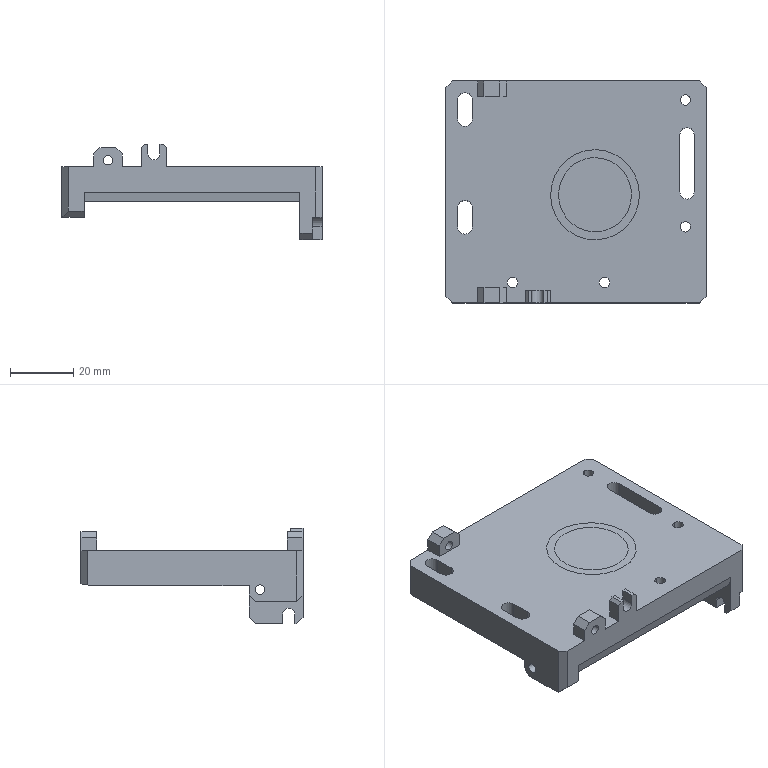NC program | NX | posted with a generic post | part box 82 x 70 x 30 mm
Lines 3883 to 5501 of 5501:
(FIXED_CONTOUR_COPY_1 , TOOL : R0.75)
N7734 T12 M6
N7736 G54
N7738 G17 G0 G90 X-35.125 Y13.063 B0. C0. S9500 M3
N7740 G43 Z30. H12
N7742 Z3.
N7744 G94 G1 Z-3.867 F1000.
N7746 X-35.098 Y13.111
N7748 X-35.049 Y13.139
N7750 X-34.995 Y13.138
N7752 X-34.959 Z-3.87 F2000.
N7754 X-34.909
N7756 X-34.892 Y13.145 Z-3.813
N7758 X-34.891 Y13.147 Z-3.801
N7760 X-34.708 Y13.148 Z-0.878
N7762 X-34.694 Z-0.85
N7764 X-31.316
N7766 X-31.288 Z-0.958
N7768 X-31.114 Y13.147 Z-3.801
N7770 X-31.092 Y13.138 Z-3.869
N7772 X-31.008 Z-3.891
N7774 X-31.092 Z-3.869
N7776 X-31.105
N7778 X-31.214 Y13.147 Z-3.801
N7780 X-31.384 Y13.148 Z-1.013
N7782 X-31.441 Z-0.95
N7784 X-34.599
N7786 X-34.631 Z-1.249
N7788 X-34.792 Y13.146 Z-3.807
N7790 X-34.809 Y13.138 Z-3.87
N7792 X-34.959
N7794 X-34.995 Z-3.868
N7796 X-34.959 Z-3.871
N7798 X-34.808 Z-3.87
N7800 X-34.692 Y13.145 Z-3.812
N7802 X-34.691 Y13.147 Z-3.801
N7804 X-34.531 Y13.148 Z-1.258
N7806 X-34.512 Z-1.077
N7808 X-34.486 Z-1.05
N7810 X-31.491
N7812 X-31.358 Y13.147 Z-3.081
N7814 X-31.314 Z-3.801
N7816 X-31.163 Y13.138 Z-3.869
N7818 X-31.092
N7820 X-31.008 Z-3.891
N7822 X-31.092 Z-3.869
N7824 X-31.33
N7826 X-31.414 Y13.147 Z-3.801
N7828 X-31.569 Y13.148 Z-1.378
N7830 X-31.595 Z-1.15
N7832 X-34.4
N7834 X-34.421 Z-1.169
N7836 X-34.431 Z-1.265
N7838 X-34.591 Y13.147 Z-3.801
N7840 X-34.599 Y13.141 Z-3.85
N7842 X-34.67 Y13.138 Z-3.87
N7844 X-34.959 Z-3.871
N7846 X-34.995 Z-3.868
N7848 X-34.959 Z-3.871
N7850 X-34.569
N7852 X-34.492 Y13.144 Z-3.819
N7854 X-34.491 Y13.147 Z-3.801
N7856 X-34.337 Y13.148 Z-1.352
N7858 X-34.318 Z-1.25
N7860 X-31.725
N7862 X-31.679 Z-1.3
N7864 X-31.547 Y13.147 Z-3.299
N7866 X-31.514 Z-3.801
N7868 X-31.379 Y13.138 Z-3.87
N7870 X-31.092
N7872 X-31.008 Z-3.891
N7874 X-31.092 Z-3.87
N7876 X-31.569
N7878 X-31.615 Y13.147 Z-3.801
N7880 X-31.765 Y13.148 Z-1.516
N7882 X-31.778 Z-1.35
N7884 X-34.224
N7886 X-34.249 Z-1.544
N7888 X-34.39 Y13.147 Z-3.801
N7890 X-34.393 Y13.143 Z-3.828
N7892 X-34.431 Y13.138 Z-3.871
N7894 X-34.959
N7896 X-34.995 Z-3.869
N7898 X-34.959 Z-3.871
N7900 X-34.33
N7902 X-34.291 Y13.145 Z-3.814
N7904 X-34.29 Y13.147 Z-3.801
N7906 X-34.149 Y13.148 Z-1.555
N7908 X-34.137 Z-1.458
N7910 X-33.954 Z-1.45
N7912 X-31.9
N7914 X-31.847 Z-1.782
N7916 X-31.715 Y13.147 Z-3.801
N7918 X-31.595 Y13.138 Z-3.87
N7920 X-31.092
N7922 X-31.008 Z-3.892
N7924 X-31.092 Z-3.87
N7926 X-31.707
N7928 X-31.807 Y13.142 Z-3.839
N7930 X-31.815 Y13.147 Z-3.801
N7932 X-31.916 Z-2.261
N7934 X-31.981 Y13.148 Z-1.572
N7936 X-31.985 Z-1.55
N7938 X-33.954
N7940 X-34.042 Z-1.554
N7942 X-34.085 Z-2.124
N7944 X-34.19 Y13.147 Z-3.801
N7946 X-34.193 Y13.143 Z-3.832
N7948 X-34.33 Y13.138 Z-3.871
N7950 X-34.96 Z-3.872
N7952 X-34.995 Z-3.869
N7954 X-34.96 Z-3.872
N7956 X-34.123 Z-3.871
N7958 X-34.099 Y13.139 Z-3.866
N7960 X-34.09 Y13.147 Z-3.8
N7962 X-34.006 Y13.148 Z-2.468
N7964 X-33.954 Z-1.726
N7966 X-33.944 Z-1.65
N7968 X-32.088
N7970 X-32.046 Z-1.95
N7972 X-31.97 Y13.147 Z-2.971
N7974 X-31.915 Z-3.801
N7976 X-31.812 Y13.138 Z-3.871
N7978 X-31.092 Z-3.87
N7980 X-31.008 Z-3.892
N7982 X-31.092 Z-3.871
N7984 X-31.869
N7986 X-32.016 Y13.147 Z-3.801
N7988 X-32.059 Z-3.136
N7990 X-32.088 Z-2.729
N7992 X-32.16 Y13.148 Z-1.856
N7994 X-32.186 Z-1.75
N7996 X-33.855
N7998 X-33.951 Z-3.192
N8000 X-33.99 Y13.147 Z-3.801
N8002 X-33.991 Y13.145 Z-3.818
N8004 X-34.091 Y13.138 Z-3.872
N8006 X-34.96
N8008 X-34.995 Z-3.869
N8010 Z-3.871
N8012 X-34.961 Z-3.874
N8014 X-33.954 Z-3.873
N8016 X-33.889 Y13.147 Z-3.801
N8018 X-33.767 Y13.148 Z-1.943
N8020 X-33.754 Z-1.85
N8022 X-32.273
N8024 X-32.258 Z-1.888
N8026 X-32.232 Z-2.203
N8028 X-32.116 Y13.147 Z-3.801
N8030 X-32.046 Y13.138 Z-3.873
N8032 X-31.092
N8034 X-31.008 Z-3.894
N8036 Z-3.896
N8038 X-31.092 Z-3.875
N8040 X-32.084
N8042 X-32.216 Y13.147 Z-3.801
N8044 X-32.284 Z-2.859
N8046 X-32.357 Y13.148 Z-1.95
N8048 X-33.657
N8050 X-33.677 Z-2.085
N8052 X-33.789 Y13.147 Z-3.8
N8054 X-33.792 Y13.144 Z-3.824
N8056 X-33.954 Y13.138 Z-3.875
N8058 X-34.963 Z-3.876
N8060 X-34.995 Z-3.874
N8062 X-34.963 Z-3.877
N8064 X-33.716 Z-3.876
N8066 X-33.691 Y13.144 Z-3.818
N8068 X-33.689 Y13.147 Z-3.801
N8070 X-33.577 Y13.148 Z-2.096
N8072 X-33.546 Z-2.05
N8074 X-32.45
N8076 X-32.357 Y13.147 Z-3.234
N8078 X-32.316 Z-3.801
N8080 X-32.284 Y13.138 Z-3.874
N8082 X-31.906 Z-3.875
N8084 X-31.092
N8086 X-31.008 Z-3.897
N8088 X-31.092 Z-3.876
N8090 X-32.302
N8092 X-32.417 Y13.147 Z-3.801
N8094 X-32.496 Z-2.741
N8096 X-32.539 Y13.148 Z-2.183
N8098 X-32.588 Z-2.15
N8100 X-33.478
N8102 X-33.536 Y13.147 Z-3.002
N8104 X-33.589 Y13.145 Z-3.81
N8106 X-33.607 Y13.138 Z-3.876
N8108 X-34.963 Y13.137 Z-3.877
N8110 X-34.995 Z-3.875
N8112 X-34.964 Z-3.878
N8114 X-33.606 Z-3.877
N8116 X-33.489 Y13.146 Z-3.808
N8118 X-33.385 Y13.147 Z-2.256
N8120 X-33.36 Z-2.25
N8122 X-32.644
N8124 X-32.53 Z-3.617
N8126 X-32.517 Z-3.801
N8128 X-32.356 Y13.138 Z-3.876
N8130 X-31.092
N8132 X-31.008 Z-3.898
N8134 X-31.092 Y13.137 Z-3.877
N8136 X-32.523
N8138 X-32.617 Y13.147 Z-3.801
N8140 X-32.724 Z-2.491
N8142 X-32.74 Z-2.35
N8144 X-33.267
N8146 X-33.294 Z-2.389
N8148 X-33.388 Z-3.801
N8150 X-33.4 Y13.14 Z-3.854
N8152 X-33.477 Y13.137 Z-3.877
N8154 X-34.964 Z-3.878
N8156 X-34.995 Z-3.876
N8158 X-34.965 Z-3.879
N8160 X-33.366 Z-3.878
N8162 X-33.29 Y13.145 Z-3.818
N8164 X-33.288 Y13.147 Z-3.801
N8166 X-33.205 Z-2.553
N8168 X-33.193 Z-2.45
N8170 X-32.841
N8172 X-32.802 Z-2.768
N8174 X-32.717 Z-3.801
N8176 X-32.573 Y13.137 Z-3.877
N8178 X-31.092
N8180 X-31.008 Z-3.899
N8182 X-31.092 Z-3.878
N8184 X-32.761
N8186 X-32.818 Y13.147 Z-3.801
N8188 X-32.906 Z-2.741
N8190 X-32.931 Z-2.55
N8192 X-33.098
N8194 X-33.128 Z-2.902
N8196 X-33.188 Z-3.801
N8198 X-33.191 Y13.143 Z-3.834
N8200 X-33.239 Y13.137 Z-3.878
N8202 X-34.965 Z-3.879
N8204 X-34.995 Z-3.877
N8206 X-34.965 Z-3.88
N8208 X-33.126 Z-3.879
N8210 X-33.089 Y13.145 Z-3.816
N8212 X-33.088 Y13.147 Z-3.801
N8214 X-33.033 Z-2.97
N8216 X-33.011 Z-2.71
N8218 X-33. Z-2.817
N8220 X-32.918 Z-3.801
N8222 X-32.791 Y13.137 Z-3.879
N8224 X-31.092 Z-3.878
N8226 X-31.008 Z-3.9
N8228 X-31.092 Z-3.878
N8230 X-32.791 Z-3.879
N8232 X-32.819 Y13.139 Z-3.862
N8234 X-33.116
N8236 X-33.126 Y13.137 Z-3.879
N8238 X-34.965 Z-3.88
N8240 X-34.995 Z-3.878
N8242 X-34.997 Y13.127 Z-3.962
N8244 X-31.092 Z-3.961
N8246 X-31.085 Z-3.962
N8248 X-31.007 Z-3.963
N8250 X-31.005 Y13.099 Z-4.058
N8252 X-31.569 Z-4.056
N8254 X-34.909 Z-4.057
N8256 X-34.999 Z-4.058
N8258 X-35. Y13.07 Z-4.154
N8260 X-34.192 Z-4.152
N8262 X-31.002 Z-4.153
N8264 Y13.053 Z-4.194
N8266 X-31.001 Y13.028 Z-4.241
N8268 X-31.012 Z-4.239
N8270 X-31.051 Z-4.243
N8272 X-34.95 Z-4.244
N8274 X-34.989 Z-4.257
N8276 X-34.999 Z-4.259
N8278 X-35. Y12.985 Z-4.338
N8280 X-34.909 Z-4.326
N8282 X-31.092
N8284 X-31.055 Z-4.322
N8286 X-31.001 Z-4.334
N8288 X-31. Y12.97 Z-4.365
N8290 X-31.001 Y12.949 Z-4.401
N8292 Y12.934 Z-4.418
N8294 X-31.078 Z-4.411
N8296 X-34.924 Y12.933
N8298 X-35. Z-4.418
N8300 Y12.87 Z-4.49
N8302 X-34.67 Z-4.488
N8304 X-31.013 Z-4.489
N8306 X-31. Z-4.49
N8308 Y12.83 Z-4.538
N8310 Y12.802 Z-4.562
N8312 X-35.
N8314 Y12.73 Z-4.631
N8316 X-34.909 Z-4.626
N8318 X-31.073
N8320 X-31. Z-4.631
N8322 X-31.001 Y12.711 Z-4.649
N8324 Y12.65 Z-4.688
N8326 X-31.03 Z-4.686
N8328 X-34.97
N8330 X-34.999 Z-4.688
N8332 X-35. Y12.593 Z-4.727
N8334 Y12.567 Z-4.741
N8336 X-31.
N8338 Y12.479 Z-4.781
N8340 X-31.087 Z-4.788
N8342 X-34.913 Y12.478
N8344 X-35. Z-4.781
N8346 Y12.387 Z-4.823
N8348 X-31.
N8350 Y12.328 Z-4.843
N8352 Y12.292 Z-4.852
N8354 X-31.092 Z-4.853
N8356 X-34.964 Z-4.854
N8358 X-35. Z-4.852
N8360 Y12.195 Z-4.876
N8362 X-34.951 Z-4.878
N8364 X-31.05
N8366 X-31. Z-4.876
N8368 Y12.119 Z-4.893
N8370 Y12.097 Z-4.894
N8372 X-35.
N8374 Y11.997 Z-4.895
N8376 X-34.911 Z-4.899
N8378 X-31.089
N8380 X-31. Z-4.895
N8382 Y11.897 Z-4.894
N8384 X-35.
N8386 Y11.881 Z-4.893
N8388 Y11.799 Z-4.874
N8390 X-34.909 Z-4.877
N8392 X-31.055
N8394 X-31. Z-4.874
N8396 Y11.703 Z-4.851
N8398 X-31.092 Z-4.852
N8400 X-34.969
N8402 X-35. Z-4.851
N8404 Y11.644 Z-4.835
N8406 Y11.608 Z-4.82
N8408 X-31.
N8410 Y11.517 Z-4.779
N8412 X-31.082 Z-4.785
N8414 X-34.918 Y11.516
N8416 X-35. Z-4.779
N8418 Y11.428 Z-4.738
N8420 X-31. Z-4.739
N8422 Y11.407 Z-4.727
N8424 X-31.001 Y11.345 Z-4.685
N8426 X-31.034 Z-4.683
N8428 X-34.965
N8430 X-34.999 Z-4.685
N8432 X-35. Y11.289 Z-4.649
N8434 Y11.266 Z-4.627
N8436 X-34.909 Z-4.622
N8438 X-31.069
N8440 X-31. Z-4.627
N8442 Y11.193 Z-4.558
N8444 X-35.
N8446 Y11.17 Z-4.538
N8448 Y11.126 Z-4.486
N8450 X-34.909 Z-4.483
N8452 X-31.016 Z-4.484
N8454 X-31. Z-4.486
N8456 X-31.001 Y11.063 Z-4.414
N8458 X-31.08 Z-4.406
N8460 X-34.92
N8462 X-35. Z-4.414
N8464 X-34.999 Y11.051 Z-4.401
N8466 X-35. Y11.029 Z-4.363
N8468 Y11.014 Z-4.332
N8470 X-34.956 Z-4.323
N8472 X-34.909 Z-4.325
N8474 X-31.092
N8476 X-31.054 Z-4.321
N8478 X-31. Z-4.332
N8480 Y10.971 Z-4.24
N8482 X-31.011 Z-4.238
N8484 X-31.05 Z-4.242
N8486 X-34.951
N8488 X-34.962 Z-4.244
N8490 X-35. Z-4.242
N8492 Y10.956 Z-4.214
N8494 Y10.933 Z-4.163
N8496 Y10.929 Z-4.152
N8498 X-34.67 Z-4.15
N8500 X-31.081 Z-4.151
N8502 X-31. Z-4.152
N8504 Y10.9 Z-4.058
N8506 X-31.092 Z-4.055
N8508 X-34.909
N8510 X-34.999 Z-4.057
N8512 X-34.996 Y10.872 Z-3.962
N8514 X-34.909 Z-3.959
N8516 X-31.081 Z-3.96
N8518 X-31.001 Z-3.963
N8520 X-31.002 Y10.859 Z-3.883
N8522 Y10.858 Z-3.867
N8524 X-31.092 Z-3.862
N8526 X-34.909 Z-3.86
N8528 X-34.925 Z-3.862
N8530 X-34.955 Z-3.873
N8532 X-34.994 Z-3.876
N8534 X-34.989 Y10.852 Z-3.776
N8536 X-34.909 Z-3.766
N8538 X-31.08 Z-3.769
N8540 X-31.065 Z-3.781
N8542 X-31.002 Z-3.786
N8544 Y10.85 Z-3.751
N8546 Z-3.686
N8548 X-31.092 Z-3.668
N8550 X-34.913 Y10.851 Z-3.666
N8552 X-34.983 Y10.85 Z-3.674
N8554 X-34.976 Z-3.573
N8556 X-34.917 Z-3.566
N8558 X-31.092 Z-3.568
N8560 X-31.002 Z-3.584
N8562 Z-3.482
N8564 X-31.092 Z-3.468
N8566 X-34.921 Y10.851 Z-3.466
N8568 X-34.97 Y10.85 Z-3.471
N8570 X-34.964 Z-3.37
N8572 X-34.925 Z-3.366
N8574 X-31.092 Z-3.368
N8576 X-31.002 Z-3.381
N8578 Z-3.28
N8580 X-31.092 Z-3.268
N8582 X-34.93 Y10.851 Z-3.266
N8584 X-34.957 Y10.85 Z-3.269
N8586 X-34.951 Z-3.168
N8588 X-34.909 Z-3.166
N8590 X-31.092 Z-3.168
N8592 X-31.002 Z-3.179
N8594 X-31.001 Z-3.078
N8596 X-31.092 Z-3.068
N8598 X-34.945 Z-3.067
N8600 X-34.941 Z-3.012
N8602 X-34.942 Z-2.985
N8604 X-34.94 Y10.849
N8606 X-34.938 Z-2.966
N8608 X-31.092 Y10.85 Z-2.968
N8610 X-31.001 Z-2.977
N8612 Z-2.876
N8614 X-31.092 Z-2.868
N8616 X-34.932 Y10.849 Z-2.866
N8618 X-34.926 Y10.85 Z-2.766
N8620 X-31.092 Z-2.768
N8622 X-31.001 Z-2.776
N8624 Z-2.675
N8626 X-31.092 Z-2.668
N8628 X-34.92 Z-2.666
N8630 X-34.913 Z-2.566
N8632 X-31.092 Z-2.568
N8634 X-31.001 Z-2.575
N8636 Z-2.475
N8638 X-31.092 Z-2.468
N8640 X-34.907 Z-2.466
N8642 X-34.901 Z-2.366
N8644 X-31.092 Z-2.368
N8646 X-31.001 Z-2.374
N8648 Z-2.274
N8650 X-31.092 Z-2.268
N8652 X-34.895 Z-2.266
N8654 X-34.888 Z-2.166
N8656 X-31.092 Z-2.168
N8658 X-31.001 Z-2.174
N8660 Z-2.073
N8662 X-31.092 Z-2.068
N8664 X-34.882 Z-2.066
N8666 X-34.876 Z-1.966
N8668 X-31.092 Z-1.968
N8670 X-31.001 Z-1.973
N8672 Z-1.873
N8674 X-31.092 Z-1.868
N8676 X-34.87 Z-1.866
N8678 X-34.863 Z-1.766
N8680 X-31.092 Z-1.768
N8682 X-31.001 Z-1.773
N8684 Z-1.672
N8686 X-31.092 Z-1.668
N8688 X-34.857 Z-1.666
N8690 X-34.851 Z-1.566
N8692 X-31.092 Z-1.568
N8694 X-31.001 Z-1.572
N8696 Z-1.472
N8698 X-31.092 Z-1.468
N8700 X-34.845 Z-1.466
N8702 X-34.838 Z-1.366
N8704 X-31.092 Z-1.368
N8706 X-31.001 Z-1.372
N8708 Z-1.272
N8710 X-31.092 Z-1.268
N8712 X-34.832 Z-1.266
N8714 X-34.826 Z-1.166
N8716 X-31.092 Z-1.168
N8718 X-31.001 Z-1.171
N8720 X-31. Z-1.071
N8722 X-31.092 Z-1.068
N8724 X-34.82 Z-1.066
N8726 X-34.813 Z-0.966
N8728 X-31.092 Z-0.968
N8730 X-31. Z-0.971
N8732 Z-0.871
N8734 X-31.088 Z-0.868
N8736 X-34.807 Z-0.866
N8738 X-34.801 Z-0.766
N8740 X-31.091 Z-0.768
N8742 X-31. Z-0.771
N8744 X-30.946 Y10.849
N8746 X-30.897 Y10.877
N8748 X-30.87 Y10.924
N8750 Z3.
N8752 G0 Z30.
N8754 M5
(ZLEVEL_PROFILE_1_COPY_1 , TOOL : D3R0.5)
N8756 T05 M6
N8758 G54
N8760 G17 G0 G90 X-35.973 Y16.812 B0. C0. S9500 M3
N8762 G43 Z30. H5
N8764 Z1.429
N8766 G94 G1 Z-0.071 F1000.
N8768 X-35.735 Y16.42
N8770 G3 X-35.472 Y16.275 R0.3
N8772 G1 X-35.35 Y16.278 F2500.
N8774 X-30.55
N8776 X-30.528 Y16.276
N8778 Y16.313 Z-0.106
N8780 Y16.347 Z-0.141
N8782 X-30.55 Y16.349
N8784 X-35.35
N8786 X-35.472 Y16.346
N8788 Y16.384 Z-0.177
N8790 Y16.417 Z-0.212
N8792 X-35. Y16.419
N8794 X-30.55
N8796 X-30.528 Y16.418
N8798 Y16.455 Z-0.247
N8800 Y16.488 Z-0.283
N8802 X-30.55 Y16.49
N8804 X-35.
N8806 X-35.472 Y16.487
N8808 Y16.525 Z-0.318
N8810 Y16.558 Z-0.354
N8812 X-35. Y16.561
N8814 X-30.55
N8816 X-30.528 Y16.559
N8818 Y16.596 Z-0.389
N8820 Y16.63 Z-0.424
N8822 X-30.55 Y16.631
N8824 X-35.
N8826 X-35.472 Y16.629
N8828 Y16.667 Z-0.46
N8830 Y16.699 Z-0.495
N8832 X-35. Y16.702
N8834 X-30.55
N8836 X-30.528 Y16.7
N8838 Y16.737 Z-0.53
N8840 Y16.771 Z-0.566
N8842 X-30.55 Y16.773
N8844 X-35.
N8846 X-35.472 Y16.77
N8848 Y16.808 Z-0.601
N8850 Y16.841 Z-0.636
N8852 X-35. Y16.844
N8854 X-30.55
N8856 X-30.528 Y16.842
N8858 Y16.879 Z-0.672
N8860 Y16.913 Z-0.707
N8862 X-30.55 Y16.914
N8864 X-35.
N8866 X-35.472 Y16.912
N8868 Y16.95 Z-0.742
N8870 Y16.982 Z-0.778
N8872 X-35. Y16.985
N8874 X-30.55
N8876 X-30.528 Y16.983
N8878 Y17.02 Z-0.813
N8880 Y17.054 Z-0.849
N8882 X-30.55 Y17.056
N8884 X-35.
N8886 X-35.472 Y17.053
N8888 Y17.091 Z-0.884
N8890 Y17.124 Z-0.919
N8892 X-35. Y17.126
N8894 X-30.55
N8896 X-30.528 Y17.125
N8898 Y17.162 Z-0.955
N8900 Y17.195 Z-0.99
N8902 X-30.55 Y17.197
N8904 X-35.
N8906 X-35.472 Y17.194
N8908 Y17.232 Z-1.025
N8910 Y17.265 Z-1.061
N8912 X-35. Y17.268
N8914 X-30.55
N8916 X-30.528 Y17.266
N8918 Y17.303 Z-1.096
N8920 Y17.337 Z-1.131
N8922 X-30.55 Y17.338
N8924 X-35.
N8926 X-35.472 Y17.336
N8928 Y17.374 Z-1.167
N8930 Y17.407 Z-1.202
N8932 X-35.35 Y17.409
N8934 X-30.55
N8936 X-30.528 Y17.408
N8938 Y17.445 Z-1.237
N8940 Y17.478 Z-1.273
N8942 X-30.55 Y17.48
N8944 X-35.35
N8946 X-35.472 Y17.477
N8948 Y17.508 Z-1.301
N8950 Y17.534 Z-1.33
N8952 X-35.35 Y17.537
N8954 X-30.55
N8956 X-30.528 Y17.535
N8958 Y17.565 Z-1.358
N8960 Y17.592 Z-1.386
N8962 X-30.55 Y17.594
N8964 X-35.35
N8966 X-35.472 Y17.591
N8968 X-35.419 Y17.648 Z-1.443
N8970 X-35.35 Y17.65
N8972 X-30.538 Y17.649
N8974 G3 X-30.278 Y17.799 R0.3
N8976 G1 X-30.052 Y18.19
N8978 Z0.057
N8980 G0 Z30.
N8982 X-29.99 Y7.198
N8984 Z1.429
N8986 G1 Z-0.071 F1000.
N8988 X-30.258 Y7.593
N8990 G3 X-30.528 Y7.724 R0.3
N8992 G1 X-30.55 Y7.722 F2500.
N8994 X-35.35
N8996 X-35.472 Y7.725
N8998 Y7.687 Z-0.106
N9000 Y7.654 Z-0.141
N9002 X-35.35 Y7.651
N9004 X-30.55
N9006 X-30.528 Y7.653
N9008 Y7.616 Z-0.177
N9010 Y7.582 Z-0.212
N9012 X-30.55 Y7.581
N9014 X-35.
N9016 X-35.472 Y7.583
N9018 Y7.545 Z-0.247
N9020 Y7.513 Z-0.283
N9022 X-35. Y7.51
N9024 X-30.55
N9026 X-30.528 Y7.512
N9028 Y7.475 Z-0.318
N9030 Y7.441 Z-0.354
N9032 X-30.55 Y7.439
N9034 X-35.
N9036 X-35.472 Y7.442
N9038 Y7.404 Z-0.389
N9040 Y7.371 Z-0.424
N9042 X-35. Y7.369
N9044 X-30.55
N9046 X-30.528 Y7.37
N9048 Y7.333 Z-0.46
N9050 Y7.3 Z-0.495
N9052 X-30.55 Y7.298
N9054 X-35.
N9056 X-35.472 Y7.301
N9058 Y7.263 Z-0.53
N9060 Y7.23 Z-0.566
N9062 X-35. Y7.227
N9064 X-30.55
N9066 X-30.528 Y7.229
N9068 Y7.192 Z-0.601
N9070 Y7.158 Z-0.636
N9072 X-30.55 Y7.156
N9074 X-35.
N9076 X-35.472 Y7.159
N9078 Y7.121 Z-0.672
N9080 Y7.088 Z-0.707
N9082 X-35. Y7.086
N9084 X-30.55
N9086 X-30.528 Y7.087
N9088 Y7.05 Z-0.742
N9090 Y7.017 Z-0.778
N9092 X-30.55 Y7.015
N9094 X-35.
N9096 X-35.472 Y7.018
N9098 Y6.98 Z-0.813
N9100 Y6.947 Z-0.849
N9102 X-35. Y6.944
N9104 X-30.55
N9106 X-30.528 Y6.946
N9108 Y6.909 Z-0.884
N9110 Y6.875 Z-0.919
N9112 X-30.55 Y6.874
N9114 X-35.
N9116 X-35.472 Y6.876
N9118 Y6.838 Z-0.955
N9120 Y6.806 Z-0.99
N9122 X-35. Y6.803
N9124 X-30.55
N9126 X-30.528 Y6.805
N9128 Y6.768 Z-1.025
N9130 Y6.734 Z-1.061
N9132 X-30.55 Y6.732
N9134 X-35.
N9136 X-35.472 Y6.735
N9138 Y6.697 Z-1.096
N9140 Y6.664 Z-1.131
N9142 X-35. Y6.662
N9144 X-30.55
N9146 X-30.528 Y6.663
N9148 Y6.626 Z-1.167
N9150 Y6.592 Z-1.202
N9152 X-30.55 Y6.591
N9154 X-35.35
N9156 X-35.472 Y6.593
N9158 Y6.555 Z-1.237
N9160 Y6.523 Z-1.273
N9162 X-35.35 Y6.52
N9164 X-30.55
N9166 X-30.528 Y6.522
N9168 Y6.492 Z-1.301
N9170 Y6.465 Z-1.33
N9172 X-30.55 Y6.463
N9174 X-35.35
N9176 X-35.472 Y6.466
N9178 Y6.435 Z-1.358
N9180 Y6.409 Z-1.386
N9182 X-35.35 Y6.406
N9184 X-30.55
N9186 X-30.528 Y6.408
N9188 X-30.533 Y6.378 Z-1.415
N9190 X-30.538 Y6.351 Z-1.443
N9192 X-35.35 Y6.35
N9194 X-35.419 Y6.352
N9196 G3 X-35.683 Y6.209 R0.3
N9198 G1 X-35.93 Y5.806
N9200 Z0.057
N9202 G0 Z30.
(ZLEVEL_PROFILE_1_COPY_1_COPY , TOOL : D3R0.5)
N9204 X28.994 Y30.803
N9206 Z0.429
N9208 G1 Z-1.071 F1000.
N9210 X29.259 Y30.408
N9212 G3 X29.528 Y30.276 R0.3
N9214 G1 X29.56 Y30.278 F2500.
N9216 X35.34
N9218 X35.472 Y30.275
N9220 Y30.313 Z-1.106
N9222 Y30.346 Z-1.141
N9224 X35.34 Y30.349
N9226 X29.56
N9228 X29.528 Y30.346
N9230 Y30.384 Z-1.177
N9232 Y30.418 Z-1.212
N9234 X30. Y30.419
N9236 X35.
N9238 X35.472 Y30.418
N9240 Y30.455 Z-1.247
N9242 Y30.488 Z-1.283
N9244 X35. Y30.49
N9246 X29.56
N9248 X29.528 Y30.488
N9250 Y30.525 Z-1.318
N9252 Y30.559 Z-1.354
N9254 X29.56 Y30.561
N9256 X35.
N9258 X35.472 Y30.558
N9260 Y30.596 Z-1.389
N9262 Y30.629 Z-1.424
N9264 X35. Y30.631
N9266 X29.56
N9268 X29.528 Y30.629
N9270 Y30.667 Z-1.46
N9272 Y30.7 Z-1.495
N9274 X29.56 Y30.702
N9276 X35.
N9278 X35.472 Y30.7
N9280 Y30.737 Z-1.53
N9282 Y30.77 Z-1.566
N9284 X35. Y30.773
N9286 X29.56
N9288 X29.528 Y30.771
N9290 Y30.808 Z-1.601
N9292 Y30.841 Z-1.636
N9294 X29.56 Y30.844
N9296 X35.
N9298 X35.472 Y30.841
N9300 Y30.879 Z-1.672
N9302 Y30.912 Z-1.707
N9304 X35. Y30.914
N9306 X29.56
N9308 X29.528 Y30.912
N9310 Y30.95 Z-1.742
N9312 Y30.983 Z-1.778
N9314 X29.56 Y30.985
N9316 X35.
N9318 X35.472 Y30.983
N9320 Y31.02 Z-1.813
N9322 Y31.053 Z-1.849
N9324 X35. Y31.056
N9326 X29.56
N9328 X29.528 Y31.053
N9330 Y31.091 Z-1.884
N9332 Y31.124 Z-1.919
N9334 X29.56 Y31.126
N9336 X35.
N9338 X35.472 Y31.124
N9340 Y31.162 Z-1.955
N9342 Y31.195 Z-1.99
N9344 X35. Y31.197
N9346 X29.56
N9348 X29.528 Y31.195
N9350 Y31.232 Z-2.025
N9352 Y31.266 Z-2.061
N9354 X29.56 Y31.268
N9356 X35.
N9358 X35.472 Y31.265
N9360 Y31.303 Z-2.096
N9362 Y31.336 Z-2.131
N9364 X35. Y31.338
N9366 X29.56
N9368 X29.528 Y31.336
N9370 Y31.374 Z-2.167
N9372 Y31.407 Z-2.202
N9374 X29.56 Y31.409
N9376 X35.
N9378 X35.472 Y31.407
N9380 Y31.445 Z-2.237
N9382 Y31.478 Z-2.273
N9384 X35. Y31.48
N9386 X29.56
N9388 X29.528 Y31.478
N9390 Y31.515 Z-2.308
N9392 Y31.548 Z-2.344
N9394 X29.56 Y31.551
N9396 X35.
N9398 X35.472 Y31.548
N9400 Y31.586 Z-2.379
N9402 Y31.619 Z-2.414
N9404 X35. Y31.621
N9406 X29.56
N9408 X29.528 Y31.619
N9410 Y31.657 Z-2.45
N9412 Y31.69 Z-2.485
N9414 X29.56 Y31.692
N9416 X35.
N9418 X35.472 Y31.69
N9420 Y31.727 Z-2.52
N9422 Y31.76 Z-2.556
N9424 X35. Y31.763
N9426 X29.56
N9428 X29.528 Y31.761
N9430 Y31.798 Z-2.591
N9432 Y31.831 Z-2.626
N9434 X29.56 Y31.833
N9436 X35.
N9438 X35.472 Y31.831
N9440 Y31.869 Z-2.662
N9442 Y31.902 Z-2.697
N9444 X35. Y31.904
N9446 X29.56
N9448 X29.528 Y31.902
N9450 Y31.94 Z-2.732
N9452 Y31.973 Z-2.768
N9454 X29.56 Y31.975
N9456 X35.
N9458 X35.472 Y31.972
N9460 Y32.01 Z-2.803
N9462 Y32.043 Z-2.838
N9464 X35. Y32.046
N9466 X29.56
N9468 X29.528 Y32.043
N9470 Y32.081 Z-2.874
N9472 Y32.114 Z-2.909
N9474 X29.56 Y32.116
N9476 X35.
N9478 X35.472 Y32.114
N9480 Y32.152 Z-2.945
N9482 Y32.185 Z-2.98
N9484 X35. Y32.187
N9486 X29.56
N9488 X29.528 Y32.185
N9490 Y32.222 Z-3.015
N9492 Y32.256 Z-3.051
N9494 X29.56 Y32.258
N9496 X35.
N9498 X35.472 Y32.255
N9500 Y32.293 Z-3.086
N9502 Y32.326 Z-3.121
N9504 X35. Y32.328
N9506 X29.56
N9508 X29.528 Y32.326
N9510 Y32.364 Z-3.157
N9512 Y32.397 Z-3.192
N9514 X29.56 Y32.399
N9516 X35.34
N9518 X35.472 Y32.397
N9520 Y32.434 Z-3.227
N9522 Y32.467 Z-3.263
N9524 X35.34 Y32.47
N9526 X29.56
N9528 X29.529 Y32.468
N9530 Y32.5 Z-3.292
N9532 Y32.527 Z-3.322
N9534 X29.56 Y32.529
N9536 X35.34
N9538 X35.472 Y32.527
N9540 Y32.559 Z-3.352
N9542 Y32.586 Z-3.381
N9544 X35.34 Y32.588
N9546 X29.56
N9548 X29.529 Y32.586
N9550 X29.541 Y32.647 Z-3.441
N9552 X29.56 Y32.648
N9554 X35.34
N9556 X35.418 Y32.646
N9558 G3 X35.681 Y32.79 R0.3
N9560 G1 X35.926 Y33.192
N9562 Z-1.941
N9564 G0 Z30.
N9566 X35.97 Y22.187
N9568 Z0.429
N9570 G1 Z-1.071 F1000.
N9572 X35.734 Y22.579
N9574 G3 X35.472 Y22.725 R0.3
N9576 G1 X35.34 Y22.722 F2500.
N9578 X29.56
N9580 X29.528 Y22.724
N9582 Y22.687 Z-1.106
N9584 Y22.654 Z-1.141
N9586 X29.56 Y22.651
N9588 X35.34
N9590 X35.472 Y22.654
N9592 Y22.616 Z-1.177
N9594 Y22.582 Z-1.212
N9596 X35. Y22.581
N9598 X30.
N9600 X29.528 Y22.582
N9602 Y22.545 Z-1.247
N9604 Y22.512 Z-1.283
N9606 X29.56 Y22.51
N9608 X35.
N9610 X35.472 Y22.512
N9612 Y22.475 Z-1.318
N9614 Y22.442 Z-1.354
N9616 X35. Y22.439
N9618 X29.56
N9620 X29.528 Y22.441
N9622 Y22.404 Z-1.389
N9624 Y22.371 Z-1.424
N9626 X29.56 Y22.369
N9628 X35.
N9630 X35.472 Y22.371
N9632 Y22.333 Z-1.46
N9634 Y22.3 Z-1.495
N9636 X35. Y22.298
N9638 X29.56
N9640 X29.528 Y22.3
N9642 Y22.263 Z-1.53
N9644 Y22.229 Z-1.566
N9646 X29.56 Y22.227
N9648 X35.
N9650 X35.472 Y22.23
N9652 Y22.192 Z-1.601
N9654 Y22.159 Z-1.636
N9656 X35. Y22.156
N9658 X29.56
N9660 X29.528 Y22.159
N9662 Y22.121 Z-1.672
N9664 Y22.088 Z-1.707
N9666 X29.56 Y22.086
N9668 X35.
N9670 X35.472 Y22.088
N9672 Y22.05 Z-1.742
N9674 Y22.017 Z-1.778
N9676 X35. Y22.015
N9678 X29.56
N9680 X29.528 Y22.017
N9682 Y21.98 Z-1.813
N9684 Y21.947 Z-1.849
N9686 X29.56 Y21.944
N9688 X35.
N9690 X35.472 Y21.947
N9692 Y21.909 Z-1.884
N9694 Y21.876 Z-1.919
N9696 X35. Y21.874
N9698 X29.56
N9700 X29.528 Y21.876
N9702 Y21.838 Z-1.955
N9704 Y21.805 Z-1.99
N9706 X29.56 Y21.803
N9708 X35.
N9710 X35.472 Y21.805
N9712 Y21.768 Z-2.025
N9714 Y21.735 Z-2.061
N9716 X35. Y21.732
N9718 X29.56
N9720 X29.528 Y21.734
N9722 Y21.697 Z-2.096
N9724 Y21.664 Z-2.131
N9726 X29.56 Y21.662
N9728 X35.
N9730 X35.472 Y21.664
N9732 Y21.626 Z-2.167
N9734 Y21.593 Z-2.202
N9736 X35. Y21.591
N9738 X29.56
N9740 X29.528 Y21.593
N9742 Y21.555 Z-2.237
N9744 Y21.522 Z-2.273
N9746 X29.56 Y21.52
N9748 X35.
N9750 X35.472 Y21.522
N9752 Y21.485 Z-2.308
N9754 Y21.452 Z-2.344
N9756 X35. Y21.449
N9758 X29.56
N9760 X29.528 Y21.452
N9762 Y21.414 Z-2.379
N9764 Y21.381 Z-2.414
N9766 X29.56 Y21.379
N9768 X35.
N9770 X35.472 Y21.381
N9772 Y21.343 Z-2.45
N9774 Y21.31 Z-2.485
N9776 X35. Y21.308
N9778 X29.56
N9780 X29.528 Y21.31
N9782 Y21.273 Z-2.52
N9784 Y21.239 Z-2.556
N9786 X29.56 Y21.237
N9788 X35.
N9790 X35.472 Y21.24
N9792 Y21.202 Z-2.591
N9794 Y21.169 Z-2.626
N9796 X35. Y21.167
N9798 X29.56
N9800 X29.528 Y21.169
N9802 Y21.131 Z-2.662
N9804 Y21.098 Z-2.697
N9806 X29.56 Y21.096
N9808 X35.
N9810 X35.472 Y21.098
N9812 Y21.06 Z-2.732
N9814 Y21.028 Z-2.768
N9816 X35. Y21.025
N9818 X29.56
N9820 X29.528 Y21.027
N9822 Y20.99 Z-2.803
N9824 Y20.957 Z-2.838
N9826 X29.56 Y20.954
N9828 X35.
N9830 X35.472 Y20.957
N9832 Y20.919 Z-2.874
N9834 Y20.886 Z-2.909
N9836 X35. Y20.884
N9838 X29.56
N9840 X29.528 Y20.886
N9842 Y20.848 Z-2.945
N9844 Y20.815 Z-2.98
N9846 X29.56 Y20.813
N9848 X35.
N9850 X35.472 Y20.815
N9852 Y20.778 Z-3.015
N9854 Y20.745 Z-3.051
N9856 X35. Y20.742
N9858 X29.56
N9860 X29.528 Y20.744
N9862 Y20.707 Z-3.086
N9864 Y20.674 Z-3.121
N9866 X29.56 Y20.672
N9868 X35.
N9870 X35.472 Y20.674
N9872 Y20.636 Z-3.157
N9874 Y20.603 Z-3.192
N9876 X35.34 Y20.601
N9878 X29.56
N9880 X29.528 Y20.603
N9882 X29.529 Y20.566 Z-3.227
N9884 Y20.532 Z-3.263
N9886 X29.56 Y20.53
N9888 X35.34
N9890 X35.472 Y20.533
N9892 Y20.5 Z-3.292
N9894 Y20.473 Z-3.322
N9896 X35.34 Y20.471
N9898 X29.56
N9900 X29.529 Y20.473
N9902 Y20.441 Z-3.352
N9904 Y20.414 Z-3.381
N9906 X29.56 Y20.412
N9908 X35.34
N9910 X35.472 Y20.414
N9912 X35.418 Y20.354 Z-3.441
N9914 X35.34 Y20.352
N9916 X29.56
N9918 X29.541 Y20.354
N9920 G3 X29.272 Y20.222 R0.3
N9922 G1 X29.003 Y19.825
N9924 Z-1.941
N9926 G0 Z30.
N9928 X-35.97 Y30.813
N9930 Z0.429
N9932 G1 Z-1.071 F1000.
N9934 X-35.734 Y30.421
N9936 G3 X-35.472 Y30.275 R0.3
N9938 G1 X-35.34 Y30.278 F2500.
N9940 X-29.56
N9942 X-29.528 Y30.276
N9944 Y30.313 Z-1.106
N9946 Y30.346 Z-1.141
N9948 X-29.56 Y30.349
N9950 X-35.34
N9952 X-35.472 Y30.346
N9954 Y30.384 Z-1.177
N9956 Y30.418 Z-1.212
N9958 X-35. Y30.419
N9960 X-30.
N9962 X-29.528 Y30.418
N9964 Y30.455 Z-1.247
N9966 Y30.488 Z-1.283
N9968 X-29.56 Y30.49
N9970 X-35.
N9972 X-35.472 Y30.488
N9974 Y30.525 Z-1.318
N9976 Y30.558 Z-1.354
N9978 X-35. Y30.561
N9980 X-29.56
N9982 X-29.528 Y30.559
N9984 Y30.596 Z-1.389
N9986 Y30.629 Z-1.424
N9988 X-29.56 Y30.631
N9990 X-35.
N9992 X-35.472 Y30.629
N9994 Y30.667 Z-1.46
N9996 Y30.7 Z-1.495
N9998 X-35. Y30.702
N10000 X-29.56
N10002 X-29.528 Y30.7
N10004 Y30.737 Z-1.53
N10006 Y30.771 Z-1.566
N10008 X-29.56 Y30.773
N10010 X-35.
N10012 X-35.472 Y30.77
N10014 Y30.808 Z-1.601
N10016 Y30.841 Z-1.636
N10018 X-35. Y30.844
N10020 X-29.56
N10022 X-29.528 Y30.841
N10024 Y30.879 Z-1.672
N10026 Y30.912 Z-1.707
N10028 X-29.56 Y30.914
N10030 X-35.
N10032 X-35.472 Y30.912
N10034 Y30.95 Z-1.742
N10036 Y30.983 Z-1.778
N10038 X-35. Y30.985
N10040 X-29.56
N10042 X-29.528 Y30.983
N10044 Y31.02 Z-1.813
N10046 Y31.053 Z-1.849
N10048 X-29.56 Y31.056
N10050 X-35.
N10052 X-35.472 Y31.053
N10054 Y31.091 Z-1.884
N10056 Y31.124 Z-1.919
N10058 X-35. Y31.126
N10060 X-29.56
N10062 X-29.528 Y31.124
N10064 Y31.162 Z-1.955
N10066 Y31.195 Z-1.99
N10068 X-29.56 Y31.197
N10070 X-35.
N10072 X-35.472 Y31.195
N10074 Y31.232 Z-2.025
N10076 Y31.265 Z-2.061
N10078 X-35. Y31.268
N10080 X-29.56
N10082 X-29.528 Y31.266
N10084 Y31.303 Z-2.096
N10086 Y31.336 Z-2.131
N10088 X-29.56 Y31.338
N10090 X-35.
N10092 X-35.472 Y31.336
N10094 X-35.473 Y31.374 Z-2.167
N10096 Y31.407 Z-2.202
N10098 X-35. Y31.409
N10100 X-29.56
N10102 X-29.528 Y31.407
N10104 Y31.445 Z-2.237
N10106 Y31.478 Z-2.273
N10108 X-29.56 Y31.48
N10110 X-35.
N10112 X-35.472 Y31.478
N10114 Y31.515 Z-2.308
N10116 Y31.548 Z-2.344
N10118 X-35. Y31.551
N10120 X-29.56
N10122 X-29.528 Y31.548
N10124 Y31.586 Z-2.379
N10126 Y31.619 Z-2.414
N10128 X-29.56 Y31.621
N10130 X-35.
N10132 X-35.472 Y31.619
N10134 Y31.657 Z-2.45
N10136 Y31.69 Z-2.485
N10138 X-35. Y31.692
N10140 X-29.56
N10142 X-29.528 Y31.69
N10144 Y31.727 Z-2.52
N10146 Y31.761 Z-2.556
N10148 X-29.56 Y31.763
N10150 X-35.
N10152 X-35.472 Y31.76
N10154 Y31.798 Z-2.591
N10156 Y31.831 Z-2.626
N10158 X-35. Y31.833
N10160 X-29.56
N10162 X-29.528 Y31.831
N10164 Y31.869 Z-2.662
N10166 Y31.902 Z-2.697
N10168 X-29.56 Y31.904
N10170 X-35.
N10172 X-35.472 Y31.902
N10174 Y31.94 Z-2.732
N10176 Y31.972 Z-2.768
N10178 X-35. Y31.975
N10180 X-29.56
N10182 X-29.528 Y31.973
N10184 Y32.01 Z-2.803
N10186 Y32.043 Z-2.838
N10188 X-29.56 Y32.046
N10190 X-35.
N10192 X-35.472 Y32.043
N10194 Y32.081 Z-2.874
N10196 Y32.114 Z-2.909
N10198 X-35. Y32.116
N10200 X-29.56
N10202 X-29.528 Y32.114
N10204 Y32.152 Z-2.945
N10206 Y32.185 Z-2.98
N10208 X-29.56 Y32.187
N10210 X-35.
N10212 X-35.472 Y32.185
N10214 Y32.222 Z-3.015
N10216 Y32.255 Z-3.051
N10218 X-35. Y32.258
N10220 X-29.56
N10222 X-29.528 Y32.256
N10224 Y32.293 Z-3.086
N10226 Y32.326 Z-3.121
N10228 X-29.56 Y32.328
N10230 X-35.
N10232 X-35.472 Y32.326
N10234 Y32.364 Z-3.157
N10236 Y32.397 Z-3.192
N10238 X-35.34 Y32.399
N10240 X-29.56
N10242 X-29.528 Y32.397
N10244 Y32.434 Z-3.227
N10246 Y32.468 Z-3.263
N10248 X-29.56 Y32.47
N10250 X-35.34
N10252 X-35.472 Y32.467
N10254 X-35.471 Y32.5 Z-3.292
N10256 Y32.527 Z-3.322
N10258 X-35.34 Y32.529
N10260 X-29.56
N10262 X-29.528 Y32.527
N10264 X-29.529 Y32.559 Z-3.352
N10266 Y32.586 Z-3.381
N10268 X-29.56 Y32.588
N10270 X-35.34
N10272 X-35.471 Y32.586
N10274 X-35.418 Y32.646 Z-3.441
N10276 X-35.34 Y32.648
N10278 X-29.56
N10280 X-29.541 Y32.646
N10282 G3 X-29.272 Y32.778 R0.3
N10284 G1 X-29.003 Y33.175
N10286 Z-1.941
N10288 G0 Z30.
N10290 X-28.994 Y22.197
N10292 Z0.429
N10294 G1 Z-1.071 F1000.
N10296 X-29.259 Y22.592
N10298 G3 X-29.528 Y22.724 R0.3
N10300 G1 X-29.56 Y22.722 F2500.
N10302 X-35.34
N10304 X-35.472 Y22.725
N10306 Y22.687 Z-1.106
N10308 Y22.654 Z-1.141
N10310 X-35.34 Y22.651
N10312 X-29.56
N10314 X-29.528 Y22.654
N10316 Y22.616 Z-1.177
N10318 Y22.582 Z-1.212
N10320 X-30. Y22.581
N10322 X-35.
N10324 X-35.472 Y22.582
N10326 Y22.545 Z-1.247
N10328 Y22.512 Z-1.283
N10330 X-35. Y22.51
N10332 X-29.56
N10334 X-29.528 Y22.512
N10336 Y22.475 Z-1.318
N10338 Y22.441 Z-1.354
N10340 X-29.56 Y22.439
N10342 X-35.
N10344 X-35.472 Y22.442
N10346 Y22.404 Z-1.389
N10348 Y22.371 Z-1.424
N10350 X-35. Y22.369
N10352 X-29.56
N10354 X-29.528 Y22.371
N10356 Y22.333 Z-1.46
N10358 Y22.3 Z-1.495
N10360 X-29.56 Y22.298
N10362 X-35.
N10364 X-35.472 Y22.3
N10366 Y22.263 Z-1.53
N10368 Y22.23 Z-1.566
N10370 X-35. Y22.227
N10372 X-29.56
N10374 X-29.528 Y22.229
N10376 Y22.192 Z-1.601
N10378 Y22.159 Z-1.636
N10380 X-29.56 Y22.156
N10382 X-35.
N10384 X-35.472 Y22.159
N10386 Y22.121 Z-1.672
N10388 Y22.088 Z-1.707
N10390 X-35. Y22.086
N10392 X-29.56
N10394 X-29.528 Y22.088
N10396 Y22.05 Z-1.742
N10398 Y22.017 Z-1.778
N10400 X-29.56 Y22.015
N10402 X-35.
N10404 X-35.472 Y22.017
N10406 Y21.98 Z-1.813
N10408 Y21.947 Z-1.849
N10410 X-35. Y21.944
N10412 X-29.56
N10414 X-29.528 Y21.947
N10416 Y21.909 Z-1.884
N10418 Y21.876 Z-1.919
N10420 X-29.56 Y21.874
N10422 X-35.
N10424 X-35.472 Y21.876
N10426 Y21.838 Z-1.955
N10428 Y21.805 Z-1.99
N10430 X-35. Y21.803
N10432 X-29.56
N10434 X-29.528 Y21.805
N10436 Y21.768 Z-2.025
N10438 Y21.734 Z-2.061
N10440 X-29.56 Y21.732
N10442 X-35.
N10444 X-35.472 Y21.735
N10446 Y21.697 Z-2.096
N10448 Y21.664 Z-2.131
N10450 X-35. Y21.662
N10452 X-29.56
N10454 X-29.528 Y21.664
N10456 Y21.626 Z-2.167
N10458 Y21.593 Z-2.202
N10460 X-29.56 Y21.591
N10462 X-35.
N10464 X-35.473 Y21.593
N10466 Y21.555 Z-2.237
N10468 X-35.472 Y21.522 Z-2.273
N10470 X-35. Y21.52
N10472 X-29.56
N10474 X-29.528 Y21.522
N10476 Y21.485 Z-2.308
N10478 Y21.452 Z-2.344
N10480 X-29.56 Y21.449
N10482 X-35.
N10484 X-35.472 Y21.452
N10486 Y21.414 Z-2.379
N10488 Y21.381 Z-2.414
N10490 X-35. Y21.379
N10492 X-29.56
N10494 X-29.528 Y21.381
N10496 Y21.343 Z-2.45
N10498 Y21.31 Z-2.485
N10500 X-29.56 Y21.308
N10502 X-35.
N10504 X-35.472 Y21.31
N10506 Y21.273 Z-2.52
N10508 Y21.24 Z-2.556
N10510 X-35. Y21.237
N10512 X-29.56
N10514 X-29.528 Y21.239
N10516 Y21.202 Z-2.591
N10518 Y21.169 Z-2.626
N10520 X-29.56 Y21.167
N10522 X-35.
N10524 X-35.472 Y21.169
N10526 Y21.131 Z-2.662
N10528 Y21.098 Z-2.697
N10530 X-35. Y21.096
N10532 X-29.56
N10534 X-29.528 Y21.098
N10536 Y21.06 Z-2.732
N10538 Y21.027 Z-2.768
N10540 X-29.56 Y21.025
N10542 X-35.
N10544 X-35.472 Y21.028
N10546 Y20.99 Z-2.803
N10548 Y20.957 Z-2.838
N10550 X-35. Y20.954
N10552 X-29.56
N10554 X-29.528 Y20.957
N10556 Y20.919 Z-2.874
N10558 Y20.886 Z-2.909
N10560 X-29.56 Y20.884
N10562 X-35.
N10564 X-35.472 Y20.886
N10566 Y20.848 Z-2.945
N10568 Y20.815 Z-2.98
N10570 X-35. Y20.813
N10572 X-29.56
N10574 X-29.528 Y20.815
N10576 Y20.778 Z-3.015
N10578 Y20.744 Z-3.051
N10580 X-29.56 Y20.742
N10582 X-35.
N10584 X-35.472 Y20.745
N10586 Y20.707 Z-3.086
N10588 Y20.674 Z-3.121
N10590 X-35. Y20.672
N10592 X-29.56
N10594 X-29.528 Y20.674
N10596 Y20.636 Z-3.157
N10598 Y20.603 Z-3.192
N10600 X-29.56 Y20.601
N10602 X-35.34
N10604 X-35.472 Y20.603
N10606 Y20.566 Z-3.227
N10608 Y20.533 Z-3.263
N10610 X-35.34 Y20.53
N10612 X-29.56
N10614 X-29.528 Y20.532
N10616 Y20.5 Z-3.292
N10618 Y20.473 Z-3.322
N10620 X-29.56 Y20.471
N10622 X-35.34
N10624 X-35.471 Y20.473
N10626 Y20.441 Z-3.352
N10628 Y20.414 Z-3.381
N10630 X-35.34 Y20.412
N10632 X-29.56
N10634 X-29.529 Y20.414
N10636 X-29.541 Y20.354 Z-3.441
N10638 X-29.56 Y20.352
N10640 X-35.34
N10642 X-35.418 Y20.354
N10644 G3 X-35.681 Y20.21 R0.3
N10646 G1 X-35.926 Y19.808
N10648 Z-1.941
N10650 G0 Z30.
N10652 M5
(PLANAR_MILL_COPY_COPY_COPY , TOOL : D6A45)
N10654 T07 M6
N10656 G54
N10658 G17 G0 G90 X28.103 Y35.3 B0. C0. S9500 M3
N10660 G43 Z30. H7
N10662 Z-6.5
N10664 G94 G1 Z-8. F1250.
N10666 X29.548 Y35.
N10668 G3 X30.414 Y34.5 R1.
N10670 X29. Y36.5 R1.5
N10672 G1 X23.
N10674 G3 X21.5 Y35. R1.5
N10676 X23. Y33.5 R1.5
N10678 G1 X27.551
N10680 G3 X27.819 Y34.463 R1.
N10682 G1 X27.661 Y35.077
N10684 Z-6.5
N10686 G0 Z30.
N10688 X-6.73 Y35.3
N10690 Z-6.5
N10692 G1 Z-8.
N10694 X-7.134 Y36.
N10696 G3 X-8. Y36.5 R1.
N10698 G1 X-11.
N10700 G3 X-12.5 Y35. R1.5
N10702 X-11. Y33.5 R1.5
N10704 G1 X-5.
N10706 G3 X-3.5 Y35. R1.5
N10708 X-5. Y36.5 R1.5
N10710 G1 X-8.
N10712 G3 X-8.866 Y36. R1.
N10714 G1 X-9.27 Y35.3
N10716 Z-6.5
N10718 G0 Z30.
N10720 X-37.191 Y35.158
N10722 Z-6.5
N10724 G1 Z-8.
N10726 X-36.757 Y34.696
N10728 G3 X-35.8 Y34.407 R1.
N10730 G1 Y38.917
N10732 G2 X-35.507 Y39.624 R1.
N10734 G1 X-33.624 Y41.507
N10736 G2 X-32.917 Y41.8 R1.
N10738 G1 X32.917
N10740 G2 X33.624 Y41.507 R1.
N10742 G1 X35.507 Y39.624
N10744 G2 X35.8 Y38.917 R1.
N10746 G1 Y34.407
N10748 G3 X36.757 Y34.696 R1.
N10750 G1 X37.191 Y35.158
N10752 Z-6.5
N10754 G0 Z30.
N10756 Y17.842
N10758 Z-6.5
N10760 G1 Z-8.
N10762 X36.757 Y18.304
N10764 G3 X35.8 Y18.593 R1.
N10766 G1 Y-38.917
N10768 G2 X35.507 Y-39.624 R1.
N10770 G1 X33.624 Y-41.507
N10772 G2 X32.917 Y-41.8 R1.
N10774 G1 X-32.917
N10776 G2 X-33.624 Y-41.507 R1.
N10778 G1 X-35.507 Y-39.624
N10780 G2 X-35.8 Y-38.917 R1.
N10782 G1 Y4.593
N10784 G3 X-36.757 Y4.304 R1.
N10786 G1 X-37.191 Y3.842
N10788 Z-6.5
N10790 G0 Z30.
N10792 X-29.35 Y-8.868
N10794 Z-6.5
N10796 G1 Y-9.228 Z-6.596
N10798 X-29.122 Y-9.622 Z-6.718
N10800 X-28.728 Y-9.85 Z-6.84
N10802 X-28.272 Z-6.963
N10804 X-27.878 Y-9.622 Z-7.085
N10806 X-27.65 Y-9.228 Z-7.207
N10808 Y-8.772 Z-7.329
N10810 X-27.878 Y-8.378 Z-7.451
N10812 X-28.272 Y-8.15 Z-7.573
N10814 X-28.728 Z-7.695
N10816 X-29.122 Y-8.378 Z-7.817
N10818 X-29.35 Y-8.772 Z-7.939
N10820 Y-9. Z-8.
N10822 G3 X-28.5 Y-9.85 R0.85
N10824 X-29.35 Y-9. R-0.85
N10826 X-29.1 Y-9.433 R0.5
N10828 G1 Z-6.5
N10830 G0 Z30.
N10832 X-11.132 Y-35.35
N10834 Z-6.5
N10836 G1 X-10.772 Z-6.596
N10838 X-10.378 Y-35.122 Z-6.718
N10840 X-10.15 Y-34.728 Z-6.84
N10842 Y-34.272 Z-6.963
N10844 X-10.378 Y-33.878 Z-7.085
N10846 X-10.772 Y-33.65 Z-7.207
N10848 X-11.228 Z-7.329
N10850 X-11.622 Y-33.878 Z-7.451
N10852 X-11.85 Y-34.272 Z-7.573
N10854 Y-34.728 Z-7.695
N10856 X-11.622 Y-35.122 Z-7.817
N10858 X-11.228 Y-35.35 Z-7.939
N10860 X-11. Z-8.
N10862 G3 X-10.15 Y-34.5 R0.85
N10864 X-11. Y-35.35 R-0.85
N10866 X-10.567 Y-35.1 R0.5
N10868 G1 Z-6.5
N10870 G0 Z30.
N10872 X7.73 Y-35.25
N10874 Z-6.5
N10876 G1 Z-8.
N10878 X8.134 Y-35.95
N10880 G3 X9. Y-36.45 R1.
N10882 G1 X18.
N10884 G3 X19.45 Y-35. R1.45
N10886 X18. Y-33.55 R1.45
N10888 G1 X0.
N10890 G3 X-1.45 Y-35. R1.45
N10892 X0. Y-36.45 R1.45
N10894 G1 X9.
N10896 G3 X9.866 Y-35.95 R1.
N10898 G1 X10.27 Y-35.25
N10900 Z-6.5
N10902 G0 Z30.
N10904 X28.868 Y-35.35
N10906 Z-6.5
N10908 G1 X29.228 Z-6.596
N10910 X29.622 Y-35.122 Z-6.718
N10912 X29.85 Y-34.728 Z-6.84
N10914 Y-34.272 Z-6.963
N10916 X29.622 Y-33.878 Z-7.085
N10918 X29.228 Y-33.65 Z-7.207
N10920 X28.772 Z-7.329
N10922 X28.378 Y-33.878 Z-7.451
N10924 X28.15 Y-34.272 Z-7.573
N10926 Y-34.728 Z-7.695
N10928 X28.378 Y-35.122 Z-7.817
N10930 X28.772 Y-35.35 Z-7.939
N10932 X29. Z-8.
N10934 G3 X29.85 Y-34.5 R0.85
N10936 X29. Y-35.35 R-0.85
N10938 X29.433 Y-35.1 R0.5
N10940 G1 Z-6.5
N10942 G0 Z30.
N10944 M5
N10946 M2